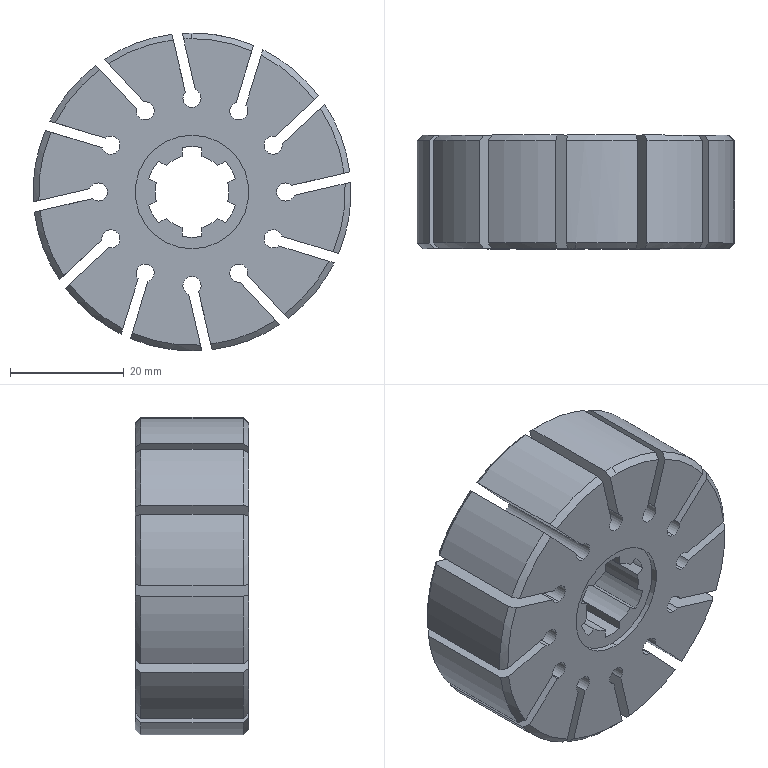Part | SolidWorks | features ICE 5, Chamfer 1, Extrusion 1 | 1 solid | 126 faces | box 56 x 20 x 56 mm | volume 39199 mm3 | cylinder 60 | plane 40 | cone 26 | commonest cylinder face diameters 3.2 x30 56 x13 16 x7 13 x6 20 x4